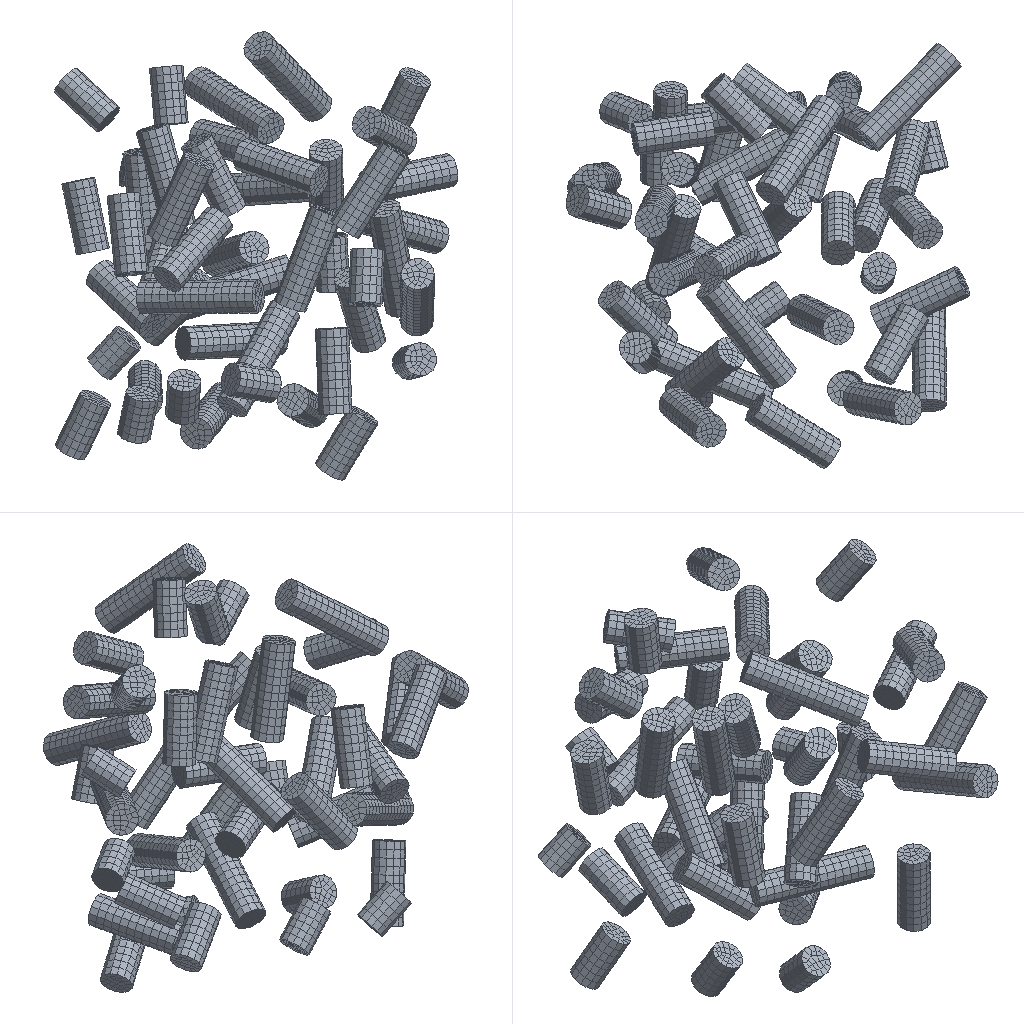Simulation study | abaqus
Set-up summary:
category,name,step,type,value,unit,region
solver,abaqus
solver,version,,,Abaqus/Explicit 2020
units,not stated in the deck,,not stated
analysis,deck,,transient,transient
load_step,Step-1,Step-1,transient,nlgeom=True
contact,interactions,,,general=1 pairs=0 ties=0
load_step,requested,,,1
mesh,nodes,,,34523
mesh,elements,,,29809
element_type,R3D3,,rigid,480
element_type,R3D4,,rigid,17507
element_type,C3D8R,,solid,11822
load,load commands in deck,,count,3
bc,support commands in deck,,count,13
material,MATERIAL-1,,in results
check,setup vs results,,match,"per instance, exact: element labels, types and connectivity; labels of the nodes the elements use; coordinates of those nodes at SINGLE_PRECISION in 4 of 4 instance(s)"
Abaqus input file, long lists of numbers shortened:
*Heading
** Job name: Job-1 Model name: Model-1
** Generated by: Abaqus/CAE 2020
*Preprint, echo=NO, model=NO, history=NO, contact=NO
**
** PARTS
**
*Part, name=par
*Node
      1,   6.853,   108.856,   37.985
      2,  -3.298,   111.792,   47.287
** (17145 more lines like these left out)
*Element, type=C3D8R
  1, 1369, 9067, 9051, 1370,  106, 1333, 1317,  107
  2, 1368, 9068, 9067, 1369,  105, 1334, 1333,  106
** (11820 more lines like these left out)
*Nset, nset=Set-1, generate
     1,  17147,      1
*Elset, elset=Set-1, generate
     1,  11822,      1
** Section: Section-1
*Solid Section, elset=Set-1, material=Material-1
,
*End Part
**
*Part, name=screw-1
*Node
      1,           0.,           0.,   6.3
      2,         267.,           0.,   6.3
** (2441 more lines like these left out)
*Element, type=R3D4
  1,    1,   33,  649,  656
  2,   33,   32,  650,  649
** (2485 more lines like these left out)
*Element, type=R3D3
1189,   33,   32, 1454
1190,   27, 1452,   28
** (104 more lines like these left out)
*Node
   2444,         277., 3.85763739e-16,           0.
*Nset, nset=screw-1-RefPt_, internal
2444,
*Elset, elset=screw-1, generate
    1,  2593,     1
*End Part
**
*Part, name=screw-2
*Node
      1,   173.233,  -99.638,       -244.5
      2,   173.233,  -99.638,         22.5
** (2419 more lines like these left out)
*Element, type=R3D4
  1,    1,   33,  649,  656
  2,   33,   32,  650,  649
** (2467 more lines like these left out)
*Element, type=R3D3
1197,  119,  120, 1454
1198,  625,  121,    3
** (96 more lines like these left out)
*Node
   2422,   179.533,  -99.638,         32.5
*Nset, nset=screw-2-RefPt_, internal
2422,
*Elset, elset=screw-2, generate
    1,  2567,     1
*End Part
**
*Part, name=shell
*Node
      1,          -5.,           0.,  -26.531
      2,          -5.,           0.,        -27.5
** (12507 more lines like these left out)
*Element, type=R3D4
 1,   1,   2, 102, 133
 2, 133, 102, 103, 132
** (12549 more lines like these left out)
*Element, type=R3D3
2737, 1294,    3, 1326
2738, 1341, 3953, 1340
** (274 more lines like these left out)
*Node
  12510,        179.5,       -137.5,         37.5
*Nset, nset=shell-RefPt_, internal
12510,
*Elset, elset=shell, generate
     1,  12827,      1
*End Part
**
**
** ASSEMBLY
**
*Assembly, name=Assembly
**
*Instance, name=par-1, part=par
          0.,         -50.,           0.
*End Instance
**
*Instance, name=screw-1-1, part=screw-1
*End Instance
**
*Instance, name=screw-2-1, part=screw-2
*End Instance
**
*Instance, name=shell-1, part=shell
*End Instance
**
*Nset, nset=Set-1, instance=par-1, generate
     1,  17147,      1
*Elset, elset=Set-1, instance=par-1, generate
     1,  11822,      1
*Nset, nset=Set-2, instance=shell-1
 12510,
*Nset, nset=Set-3, instance=screw-1-1
 2444,
*Nset, nset=Set-4, instance=screw-2-1
 2422,
*Nset, nset=Set-5, instance=par-1, generate
     1,  17147,      1
*Elset, elset=Set-5, instance=par-1, generate
     1,  11822,      1
*Rigid Body, ref node=screw-1-1.screw-1-RefPt_, elset=screw-1-1.screw-1
*Rigid Body, ref node=screw-2-1.screw-2-RefPt_, elset=screw-2-1.screw-2
*Rigid Body, ref node=shell-1.shell-RefPt_, elset=shell-1.shell
*End Assembly
**
** MATERIALS
**
*Material, name=Material-1
*Density
 2.7e-09,
*Elastic
11000., 0.3
**
** INTERACTION PROPERTIES
**
*Surface Interaction, name=IntProp-1
*Friction
 0.1,
*Surface Behavior, pressure-overclosure=HARD
** ----------------------------------------------------------------
**
** STEP: Step-1
**
*Step, name=Step-1, nlgeom=YES
*Dynamic, Explicit
, 0.1
*Bulk Viscosity
0.06, 1.2
**
** BOUNDARY CONDITIONS
**
** Name: BC-1 Type: 对称/反对称/完全固定
*Boundary
Set-2, ENCASTRE
** Name: BC-3 Type: 速度/角速度
*Boundary, type=VELOCITY
Set-4, 1, 1
Set-4, 2, 2
Set-4, 3, 3
Set-4, 4, 4
Set-4, 5, 5
Set-4, 6, 6, -44.
** Name: [REDACTED] : Velocity/Angular velocity
*Boundary, type=VELOCITY
Set-3, 1, 1
Set-3, 2, 2
Set-3, 3, 3
Set-3, 4, 4, -44.
Set-3, 5, 5
Set-3, 6, 6
**
** LOADS
**
** Name: Load-1   Type: Gravity
*Dload
Set-1, GRAV, 25800., 0., -1., 0.
**
** INTERACTIONS
**
** Interaction: Int-1
*Contact, op=NEW
*Contact Inclusions, ALL EXTERIOR
*Contact Property Assignment
 ,  , IntProp-1
**
** OUTPUT REQUESTS
**
*Restart, write, number interval=1, time marks=NO
**
** FIELD OUTPUT: F-Output-1
**
*Output, field, number interval=50
*Node Output
A, RF, U, V
*Element Output, directions=YES
E, EVF, LE, MISES, MISESMAX, PE, PEEQ, PEEQVAVG, PEVAVG, S, SVAVG
*Contact Output
CSTRESS,
**
** HISTORY OUTPUT: H-Output-1
**
*Output, history, variable=PRESELECT
*End Step
Results summary:
result,step,Step-1,completed,increments=230184 time=0.1/0.1
result,analysis,,,transient
result,last_loadstep,,,1
result,analysis steps,,count,1
result,primary field,,,U
result,reaction total,,FX,-5.473,model units
result,reaction total,,FY,0.0,model units
result,reaction total,,FZ,0.1035,model units